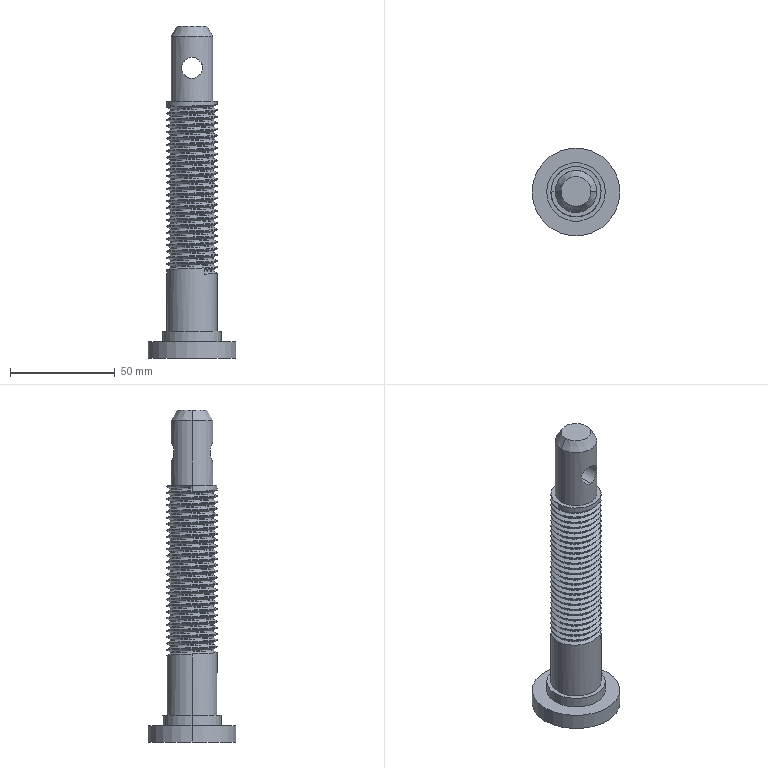Part | SolidWorks | features ICE 4, Chamfer 1, Extrusion 1, SweepThread 1 | 1 solid | 75 faces | box 42 x 42 x 158.7 mm | volume 67679 mm3 | cylinder 63 | plane 7 | spline 3 | cone 2 | commonest cylinder face diameters 24 x55 10 x2 20 x2 28 x2 42 x2